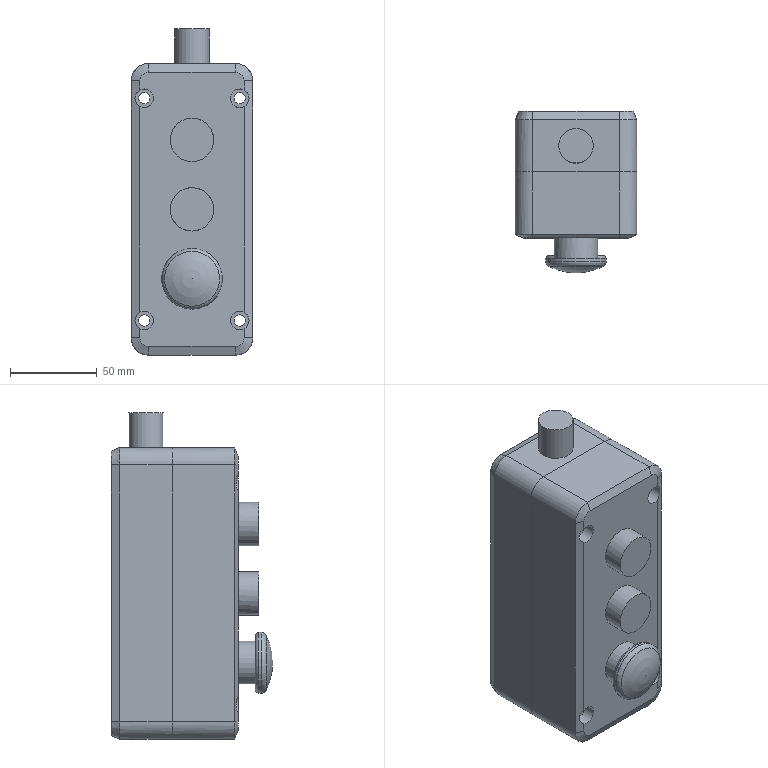Part | STEP file | Button box | 1 solid | 58 faces | box 70 x 93 x 188 mm | volume 866675 mm3 | plane 26 | cylinder 21 | cone 8 | torus 2 | sphere 1 | commonest cylinder face diameters 20 x9 6.5 x4 10.7 x4 25 x3 35 x1